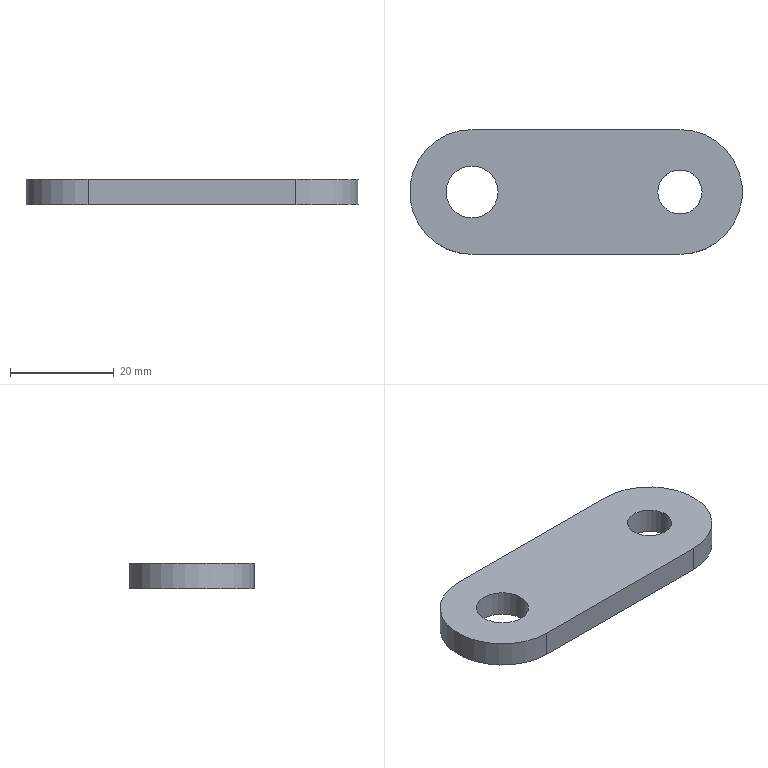Part | NX | features DATUM_CSYS 1, EXTRACT_DATUM_PLANE 1, EXTRUDE 1, SKETCH 1 | 1 solid | 8 faces | box 64 x 24 x 5 mm | volume 6386 mm3 | plane 4 | cylinder 4 | commonest cylinder face diameters 24 x2 8.5 x1 10 x1
STEP:
#1=CARTESIAN_POINT('',(0.,-12.,0.));
#2=VERTEX_POINT('',#1);
#3=CARTESIAN_POINT('',(40.,-12.,0.));
#4=VERTEX_POINT('',#3);
#5=CARTESIAN_POINT('',(0.,-12.,0.));
#6=DIRECTION('',(1.,0.,0.));
#7=VECTOR('',#6,1000.);
#8=LINE('',#5,#7);
#9=EDGE_CURVE('',#2,#4,#8,.T.);
#10=ORIENTED_EDGE('',*,*,#9,.T.);
#11=CARTESIAN_POINT('',(40.,-12.,5.));
#12=VERTEX_POINT('',#11);
#13=CARTESIAN_POINT('',(40.,-12.,5.));
#14=DIRECTION('',(0.,0.,-1.));
#15=VECTOR('',#14,1000.);
#16=LINE('',#13,#15);
#17=EDGE_CURVE('',#12,#4,#16,.T.);
#18=ORIENTED_EDGE('',*,*,#17,.F.);
#19=CARTESIAN_POINT('',(0.,-12.,5.));
#20=VERTEX_POINT('',#19);
#21=CARTESIAN_POINT('',(0.,-12.,5.));
#22=DIRECTION('',(1.,0.,0.));
#23=VECTOR('',#22,1000.);
#24=LINE('',#21,#23);
#25=EDGE_CURVE('',#20,#12,#24,.T.);
#26=ORIENTED_EDGE('',*,*,#25,.F.);
#27=CARTESIAN_POINT('',(0.,-12.,5.));
#28=DIRECTION('',(0.,0.,-1.));
#29=VECTOR('',#28,1000.);
#30=LINE('',#27,#29);
#31=EDGE_CURVE('',#20,#2,#30,.T.);
#32=ORIENTED_EDGE('',*,*,#31,.T.);
#33=EDGE_LOOP('',(#10,#18,#26,#32));
#34=FACE_BOUND('',#33,.T.);
#35=CARTESIAN_POINT('',(0.,-12.,5.));
#36=DIRECTION('',(0.,1.,0.));
#37=DIRECTION('',(0.,0.,1.));
#38=AXIS2_PLACEMENT_3D('',#35,#36,#37);
#39=PLANE('',#38);
#40=ADVANCED_FACE('',(#34),#39,.F.);
#41=CARTESIAN_POINT('',(40.,12.,0.));
#42=VERTEX_POINT('',#41);
#43=CARTESIAN_POINT('',(40.,0.,0.));
#44=DIRECTION('',(0.,0.,1.));
#45=DIRECTION('',(0.,-1.,0.));
#46=AXIS2_PLACEMENT_3D('',#43,#44,#45);
#47=CIRCLE('',#46,12.);
#48=EDGE_CURVE('',#4,#42,#47,.T.);
#49=ORIENTED_EDGE('',*,*,#48,.T.);
#50=CARTESIAN_POINT('',(40.,12.,5.));
#51=VERTEX_POINT('',#50);
#52=CARTESIAN_POINT('',(40.,12.,5.));
#53=DIRECTION('',(0.,0.,-1.));
#54=VECTOR('',#53,1000.);
#55=LINE('',#52,#54);
#56=EDGE_CURVE('',#51,#42,#55,.T.);
#57=ORIENTED_EDGE('',*,*,#56,.F.);
#58=CARTESIAN_POINT('',(40.,0.,5.));
#59=DIRECTION('',(0.,0.,1.));
#60=DIRECTION('',(0.,-1.,0.));
#61=AXIS2_PLACEMENT_3D('',#58,#59,#60);
#62=CIRCLE('',#61,12.);
#63=EDGE_CURVE('',#12,#51,#62,.T.);
#64=ORIENTED_EDGE('',*,*,#63,.F.);
#65=ORIENTED_EDGE('',*,*,#17,.T.);
#66=EDGE_LOOP('',(#49,#57,#64,#65));
#67=FACE_BOUND('',#66,.T.);
#68=CARTESIAN_POINT('',(40.,0.,5.));
#69=DIRECTION('',(0.,0.,-1.));
#70=DIRECTION('',(-1.,0.,0.));
#71=AXIS2_PLACEMENT_3D('',#68,#69,#70);
#72=CYLINDRICAL_SURFACE('',#71,12.);
#73=ADVANCED_FACE('',(#67),#72,.T.);
#74=CARTESIAN_POINT('',(0.,12.,0.));
#75=VERTEX_POINT('',#74);
#76=CARTESIAN_POINT('',(40.,12.,0.));
#77=DIRECTION('',(-1.,0.,0.));
#78=VECTOR('',#77,1000.);
#79=LINE('',#76,#78);
#80=EDGE_CURVE('',#42,#75,#79,.T.);
#81=ORIENTED_EDGE('',*,*,#80,.T.);
#82=CARTESIAN_POINT('',(0.,12.,5.));
#83=VERTEX_POINT('',#82);
#84=CARTESIAN_POINT('',(0.,12.,5.));
#85=DIRECTION('',(0.,0.,-1.));
#86=VECTOR('',#85,1000.);
#87=LINE('',#84,#86);
#88=EDGE_CURVE('',#83,#75,#87,.T.);
#89=ORIENTED_EDGE('',*,*,#88,.F.);
#90=CARTESIAN_POINT('',(40.,12.,5.));
#91=DIRECTION('',(-1.,0.,0.));
#92=VECTOR('',#91,1000.);
#93=LINE('',#90,#92);
#94=EDGE_CURVE('',#51,#83,#93,.T.);
#95=ORIENTED_EDGE('',*,*,#94,.F.);
#96=ORIENTED_EDGE('',*,*,#56,.T.);
#97=EDGE_LOOP('',(#81,#89,#95,#96));
#98=FACE_BOUND('',#97,.T.);
#99=CARTESIAN_POINT('',(40.,12.,5.));
#100=DIRECTION('',(0.,-1.,0.));
#101=DIRECTION('',(0.,0.,-1.));
#102=AXIS2_PLACEMENT_3D('',#99,#100,#101);
#103=PLANE('',#102);
#104=ADVANCED_FACE('',(#98),#103,.F.);
#105=CARTESIAN_POINT('',(-5.,0.,0.));
#106=VERTEX_POINT('',#105);
#107=CARTESIAN_POINT('',(0.,0.,0.));
#108=DIRECTION('',(0.,0.,-1.));
#109=DIRECTION('',(-1.,0.,0.));
#110=AXIS2_PLACEMENT_3D('',#107,#108,#109);
#111=CIRCLE('',#110,5.);
#112=EDGE_CURVE('',#106,#106,#111,.T.);
#113=ORIENTED_EDGE('',*,*,#112,.T.);
#114=EDGE_LOOP('',(#113));
#115=FACE_BOUND('',#114,.T.);
#116=CARTESIAN_POINT('',(5.,0.,5.));
#117=VERTEX_POINT('',#116);
#118=CARTESIAN_POINT('',(0.,0.,5.));
#119=DIRECTION('',(0.,0.,-1.));
#120=DIRECTION('',(1.,0.,0.));
#121=AXIS2_PLACEMENT_3D('',#118,#119,#120);
#122=CIRCLE('',#121,5.);
#123=EDGE_CURVE('',#117,#117,#122,.T.);
#124=ORIENTED_EDGE('',*,*,#123,.F.);
#125=EDGE_LOOP('',(#124));
#126=FACE_BOUND('',#125,.T.);
#127=CARTESIAN_POINT('',(0.,0.,5.));
#128=DIRECTION('',(0.,0.,-1.));
#129=DIRECTION('',(-1.,0.,0.));
#130=AXIS2_PLACEMENT_3D('',#127,#128,#129);
#131=CYLINDRICAL_SURFACE('',#130,5.);
#132=ADVANCED_FACE('',(#115,#126),#131,.F.);
#133=CARTESIAN_POINT('',(0.,0.,0.));
#134=DIRECTION('',(0.,0.,1.));
#135=DIRECTION('',(0.,1.,0.));
#136=AXIS2_PLACEMENT_3D('',#133,#134,#135);
#137=CIRCLE('',#136,12.);
#138=EDGE_CURVE('',#75,#2,#137,.T.);
#139=ORIENTED_EDGE('',*,*,#138,.T.);
#140=ORIENTED_EDGE('',*,*,#31,.F.);
#141=CARTESIAN_POINT('',(0.,0.,5.));
#142=DIRECTION('',(0.,0.,1.));
#143=DIRECTION('',(-1.,0.,0.));
#144=AXIS2_PLACEMENT_3D('',#141,#142,#143);
#145=CIRCLE('',#144,12.);
#146=EDGE_CURVE('',#83,#20,#145,.T.);
#147=ORIENTED_EDGE('',*,*,#146,.F.);
#148=ORIENTED_EDGE('',*,*,#88,.T.);
#149=EDGE_LOOP('',(#139,#140,#147,#148));
#150=FACE_BOUND('',#149,.T.);
#151=CARTESIAN_POINT('',(0.,0.,5.));
#152=DIRECTION('',(0.,0.,-1.));
#153=DIRECTION('',(-1.,0.,0.));
#154=AXIS2_PLACEMENT_3D('',#151,#152,#153);
#155=CYLINDRICAL_SURFACE('',#154,12.);
#156=ADVANCED_FACE('',(#150),#155,.T.);
#157=CARTESIAN_POINT('',(35.75,0.,0.));
#158=VERTEX_POINT('',#157);
#159=CARTESIAN_POINT('',(40.,0.,0.));
#160=DIRECTION('',(0.,0.,-1.));
#161=DIRECTION('',(-1.,0.,0.));
#162=AXIS2_PLACEMENT_3D('',#159,#160,#161);
#163=CIRCLE('',#162,4.25);
#164=EDGE_CURVE('',#158,#158,#163,.T.);
#165=ORIENTED_EDGE('',*,*,#164,.T.);
#166=EDGE_LOOP('',(#165));
#167=FACE_BOUND('',#166,.T.);
#168=CARTESIAN_POINT('',(44.25,0.,5.));
#169=VERTEX_POINT('',#168);
#170=CARTESIAN_POINT('',(40.,0.,5.));
#171=DIRECTION('',(0.,0.,-1.));
#172=DIRECTION('',(1.,0.,0.));
#173=AXIS2_PLACEMENT_3D('',#170,#171,#172);
#174=CIRCLE('',#173,4.25);
#175=EDGE_CURVE('',#169,#169,#174,.T.);
#176=ORIENTED_EDGE('',*,*,#175,.F.);
#177=EDGE_LOOP('',(#176));
#178=FACE_BOUND('',#177,.T.);
#179=CARTESIAN_POINT('',(40.,0.,5.));
#180=DIRECTION('',(0.,0.,-1.));
#181=DIRECTION('',(-1.,0.,0.));
#182=AXIS2_PLACEMENT_3D('',#179,#180,#181);
#183=CYLINDRICAL_SURFACE('',#182,4.25);
#184=ADVANCED_FACE('',(#167,#178),#183,.F.);
#185=ORIENTED_EDGE('',*,*,#146,.T.);
#186=ORIENTED_EDGE('',*,*,#25,.T.);
#187=ORIENTED_EDGE('',*,*,#63,.T.);
#188=ORIENTED_EDGE('',*,*,#94,.T.);
#189=EDGE_LOOP('',(#185,#186,#187,#188));
#190=FACE_BOUND('',#189,.T.);
#191=ORIENTED_EDGE('',*,*,#123,.T.);
#192=EDGE_LOOP('',(#191));
#193=FACE_BOUND('',#192,.T.);
#194=ORIENTED_EDGE('',*,*,#175,.T.);
#195=EDGE_LOOP('',(#194));
#196=FACE_BOUND('',#195,.T.);
#197=CARTESIAN_POINT('',(0.,0.,5.));
#198=DIRECTION('',(0.,0.,1.));
#199=DIRECTION('',(1.,0.,0.));
#200=AXIS2_PLACEMENT_3D('',#197,#198,#199);
#201=PLANE('',#200);
#202=ADVANCED_FACE('',(#190,#193,#196),#201,.T.);
#203=ORIENTED_EDGE('',*,*,#9,.F.);
#204=ORIENTED_EDGE('',*,*,#138,.F.);
#205=ORIENTED_EDGE('',*,*,#80,.F.);
#206=ORIENTED_EDGE('',*,*,#48,.F.);
#207=EDGE_LOOP('',(#203,#204,#205,#206));
#208=FACE_BOUND('',#207,.T.);
#209=ORIENTED_EDGE('',*,*,#112,.F.);
#210=EDGE_LOOP('',(#209));
#211=FACE_BOUND('',#210,.T.);
#212=ORIENTED_EDGE('',*,*,#164,.F.);
#213=EDGE_LOOP('',(#212));
#214=FACE_BOUND('',#213,.T.);
#215=CARTESIAN_POINT('',(0.,0.,0.));
#216=DIRECTION('',(0.,0.,1.));
#217=DIRECTION('',(1.,0.,0.));
#218=AXIS2_PLACEMENT_3D('',#215,#216,#217);
#219=PLANE('',#218);
#220=ADVANCED_FACE('',(#208,#211,#214),#219,.F.);
#221=CLOSED_SHELL('',(#40,#73,#104,#132,#156,#184,#202,#220));
#222=MANIFOLD_SOLID_BREP('',#221);
#223=(LENGTH_UNIT()NAMED_UNIT(*)SI_UNIT(.MILLI.,.METRE.));
#224=UNCERTAINTY_MEASURE_WITH_UNIT(LENGTH_MEASURE(0.00001),#223,'','');
#225=(NAMED_UNIT(*)PLANE_ANGLE_UNIT()SI_UNIT($,.RADIAN.));
#226=(NAMED_UNIT(*)SI_UNIT($,.STERADIAN.)SOLID_ANGLE_UNIT());
#227=(GEOMETRIC_REPRESENTATION_CONTEXT(3)GLOBAL_UNCERTAINTY_ASSIGNED_CONTEXT((#224))GLOBAL_UNIT_ASSIGNED_CONTEXT((#223,#225,#226))REPRESENTATION_CONTEXT('',''));
#228=ADVANCED_BREP_SHAPE_REPRESENTATION('',(#222),#227);